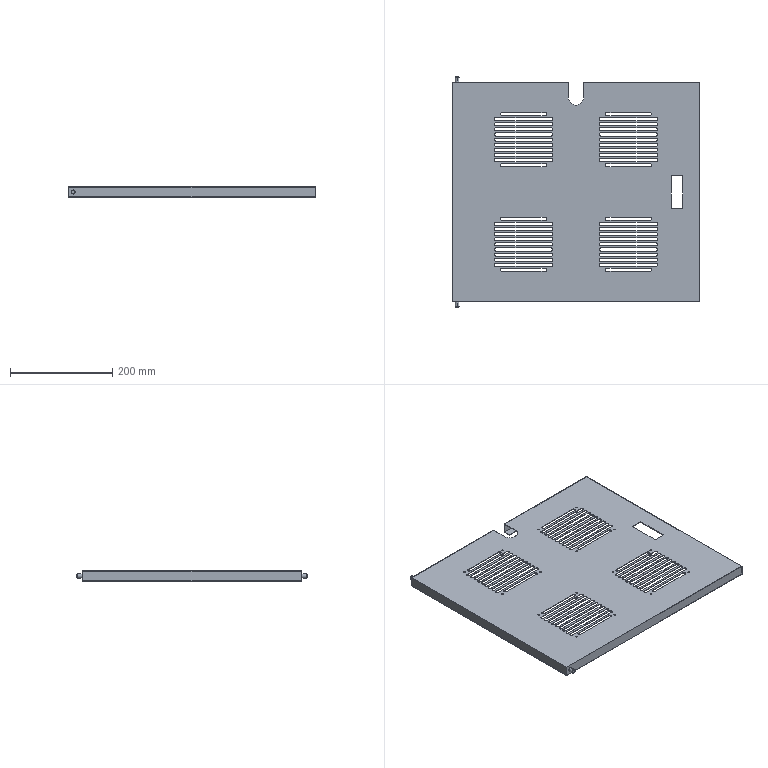Part | SolidWorks | features ICE 14, LPattern 4, Chamfer 3, Fillet 2, MirrorPattern 2, Extrusion 1, Shell 1 | 1 solid | 312 faces | box 485 x 450 x 20 mm | volume 237812 mm3 | cylinder 177 | plane 131 | cone 4 | commonest cylinder face diameters 6 x140 3 x32 8 x4 30 x1